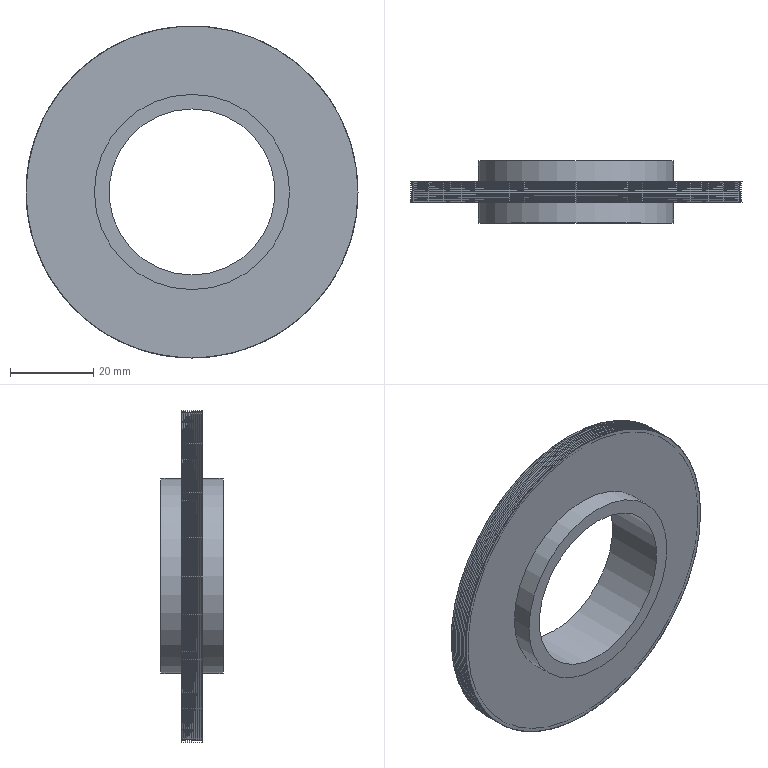Part | NX | features DATUM_CSYS 5, SKETCH 4, EXTRUDE 3, SWP104 1 | 1 solid | 41 faces | box 80 x 15 x 80 mm | volume 23126 mm3 | cone 22 | cylinder 15 | plane 4 | commonest cylinder face diameters 80 x12 47 x2 40 x1
STEP:
#1=CARTESIAN_POINT('',(40.,-10.,0.));
#2=VERTEX_POINT('',#1);
#3=CARTESIAN_POINT('',(0.,-10.,0.));
#4=DIRECTION('',(0.,1.,0.));
#5=DIRECTION('',(1.,0.,0.));
#6=AXIS2_PLACEMENT_3D('',#3,#4,#5);
#7=CIRCLE('',#6,40.);
#8=EDGE_CURVE('',#2,#2,#7,.T.);
#9=ORIENTED_EDGE('',*,*,#8,.T.);
#10=EDGE_LOOP('',(#9));
#11=FACE_BOUND('',#10,.T.);
#12=CARTESIAN_POINT('',(0.,-9.976,-40.));
#13=VERTEX_POINT('',#12);
#14=CARTESIAN_POINT('',(0.,-9.976,0.));
#15=DIRECTION('',(0.,-1.,0.));
#16=DIRECTION('',(0.,0.,-1.));
#17=AXIS2_PLACEMENT_3D('',#14,#15,#16);
#18=CIRCLE('',#17,40.);
#19=EDGE_CURVE('',#13,#13,#18,.T.);
#20=ORIENTED_EDGE('',*,*,#19,.T.);
#21=EDGE_LOOP('',(#20));
#22=FACE_BOUND('',#21,.T.);
#23=CARTESIAN_POINT('',(0.,-10.,0.));
#24=DIRECTION('',(0.,1.,0.));
#25=DIRECTION('',(0.,0.,1.));
#26=AXIS2_PLACEMENT_3D('',#23,#24,#25);
#27=CYLINDRICAL_SURFACE('',#26,40.);
#28=ADVANCED_FACE('',(#11,#22),#27,.T.);
#29=CARTESIAN_POINT('',(23.5,-15.,0.));
#30=VERTEX_POINT('',#29);
#31=CARTESIAN_POINT('',(0.,-15.,0.));
#32=DIRECTION('',(0.,-1.,0.));
#33=DIRECTION('',(1.,0.,0.));
#34=AXIS2_PLACEMENT_3D('',#31,#32,#33);
#35=CIRCLE('',#34,23.5);
#36=EDGE_CURVE('',#30,#30,#35,.T.);
#37=ORIENTED_EDGE('',*,*,#36,.F.);
#38=EDGE_LOOP('',(#37));
#39=FACE_BOUND('',#38,.T.);
#40=CARTESIAN_POINT('',(0.,-10.,23.5));
#41=VERTEX_POINT('',#40);
#42=CARTESIAN_POINT('',(0.,-10.,0.));
#43=DIRECTION('',(0.,1.,0.));
#44=DIRECTION('',(0.,0.,1.));
#45=AXIS2_PLACEMENT_3D('',#42,#43,#44);
#46=CIRCLE('',#45,23.5);
#47=EDGE_CURVE('',#41,#41,#46,.T.);
#48=ORIENTED_EDGE('',*,*,#47,.F.);
#49=EDGE_LOOP('',(#48));
#50=FACE_BOUND('',#49,.T.);
#51=CARTESIAN_POINT('',(0.,-15.,0.));
#52=DIRECTION('',(0.,1.,0.));
#53=DIRECTION('',(0.,0.,1.));
#54=AXIS2_PLACEMENT_3D('',#51,#52,#53);
#55=CYLINDRICAL_SURFACE('',#54,23.5);
#56=ADVANCED_FACE('',(#39,#50),#55,.T.);
#57=CARTESIAN_POINT('',(0.,-15.,-20.));
#58=VERTEX_POINT('',#57);
#59=CARTESIAN_POINT('',(0.,-15.,0.));
#60=DIRECTION('',(0.,-1.,0.));
#61=DIRECTION('',(0.,0.,-1.));
#62=AXIS2_PLACEMENT_3D('',#59,#60,#61);
#63=CIRCLE('',#62,20.);
#64=EDGE_CURVE('',#58,#58,#63,.F.);
#65=ORIENTED_EDGE('',*,*,#64,.T.);
#66=EDGE_LOOP('',(#65));
#67=FACE_BOUND('',#66,.T.);
#68=ORIENTED_EDGE('',*,*,#36,.T.);
#69=EDGE_LOOP('',(#68));
#70=FACE_BOUND('',#69,.T.);
#71=CARTESIAN_POINT('',(0.,-15.,0.));
#72=DIRECTION('',(0.,-1.,0.));
#73=DIRECTION('',(0.,0.,-1.));
#74=AXIS2_PLACEMENT_3D('',#71,#72,#73);
#75=PLANE('',#74);
#76=ADVANCED_FACE('',(#67,#70),#75,.T.);
#77=ORIENTED_EDGE('',*,*,#47,.T.);
#78=EDGE_LOOP('',(#77));
#79=FACE_BOUND('',#78,.T.);
#80=ORIENTED_EDGE('',*,*,#8,.F.);
#81=EDGE_LOOP('',(#80));
#82=FACE_BOUND('',#81,.T.);
#83=CARTESIAN_POINT('',(0.,-10.,0.));
#84=DIRECTION('',(0.,1.,0.));
#85=DIRECTION('',(0.,0.,1.));
#86=AXIS2_PLACEMENT_3D('',#83,#84,#85);
#87=PLANE('',#86);
#88=ADVANCED_FACE('',(#79,#82),#87,.F.);
#89=ORIENTED_EDGE('',*,*,#19,.F.);
#90=EDGE_LOOP('',(#89));
#91=FACE_BOUND('',#90,.T.);
#92=CARTESIAN_POINT('',(0.,-9.892,-39.157));
#93=VERTEX_POINT('',#92);
#94=CARTESIAN_POINT('',(0.,-9.892,0.));
#95=DIRECTION('',(0.,-1.,0.));
#96=DIRECTION('',(0.,0.,-1.));
#97=AXIS2_PLACEMENT_3D('',#94,#95,#96);
#98=CIRCLE('',#97,39.157);
#99=EDGE_CURVE('',#93,#93,#98,.F.);
#100=ORIENTED_EDGE('',*,*,#99,.F.);
#101=EDGE_LOOP('',(#100));
#102=FACE_BOUND('',#101,.T.);
#103=CARTESIAN_POINT('',(0.,-10.,0.));
#104=DIRECTION('',(0.,-1.,0.));
#105=DIRECTION('',(0.,0.,-1.));
#106=AXIS2_PLACEMENT_3D('',#103,#104,#105);
#107=CONICAL_SURFACE('',#106,40.237,1.471);
#108=ADVANCED_FACE('',(#91,#102),#107,.T.);
#109=CARTESIAN_POINT('',(0.,-9.682,40.));
#110=VERTEX_POINT('',#109);
#111=CARTESIAN_POINT('',(0.,-9.682,0.));
#112=DIRECTION('',(0.,1.,0.));
#113=DIRECTION('',(0.,0.,1.));
#114=AXIS2_PLACEMENT_3D('',#111,#112,#113);
#115=CIRCLE('',#114,40.);
#116=EDGE_CURVE('',#110,#110,#115,.T.);
#117=ORIENTED_EDGE('',*,*,#116,.F.);
#118=EDGE_LOOP('',(#117));
#119=FACE_BOUND('',#118,.T.);
#120=ORIENTED_EDGE('',*,*,#99,.T.);
#121=EDGE_LOOP('',(#120));
#122=FACE_BOUND('',#121,.T.);
#123=CARTESIAN_POINT('',(0.,-9.892,0.));
#124=DIRECTION('',(0.,1.,0.));
#125=DIRECTION('',(0.,0.,1.));
#126=AXIS2_PLACEMENT_3D('',#123,#124,#125);
#127=CONICAL_SURFACE('',#126,39.157,1.326);
#128=ADVANCED_FACE('',(#119,#122),#127,.T.);
#129=CARTESIAN_POINT('',(0.,-9.67,-40.));
#130=VERTEX_POINT('',#129);
#131=CARTESIAN_POINT('',(0.,-9.67,0.));
#132=DIRECTION('',(0.,-1.,0.));
#133=DIRECTION('',(0.,0.,-1.));
#134=AXIS2_PLACEMENT_3D('',#131,#132,#133);
#135=CIRCLE('',#134,40.);
#136=EDGE_CURVE('',#130,#130,#135,.T.);
#137=ORIENTED_EDGE('',*,*,#136,.T.);
#138=EDGE_LOOP('',(#137));
#139=FACE_BOUND('',#138,.T.);
#140=ORIENTED_EDGE('',*,*,#116,.T.);
#141=EDGE_LOOP('',(#140));
#142=FACE_BOUND('',#141,.T.);
#143=CARTESIAN_POINT('',(0.,-10.,0.));
#144=DIRECTION('',(0.,1.,0.));
#145=DIRECTION('',(0.,0.,1.));
#146=AXIS2_PLACEMENT_3D('',#143,#144,#145);
#147=CYLINDRICAL_SURFACE('',#146,40.);
#148=ADVANCED_FACE('',(#139,#142),#147,.T.);
#149=CARTESIAN_POINT('',(0.,-9.218,40.));
#150=VERTEX_POINT('',#149);
#151=CARTESIAN_POINT('',(0.,-9.218,0.));
#152=DIRECTION('',(0.,1.,0.));
#153=DIRECTION('',(0.,0.,1.));
#154=AXIS2_PLACEMENT_3D('',#151,#152,#153);
#155=CIRCLE('',#154,40.);
#156=EDGE_CURVE('',#150,#150,#155,.T.);
#157=ORIENTED_EDGE('',*,*,#156,.F.);
#158=EDGE_LOOP('',(#157));
#159=FACE_BOUND('',#158,.T.);
#160=CARTESIAN_POINT('',(0.,-9.428,-39.157));
#161=VERTEX_POINT('',#160);
#162=CARTESIAN_POINT('',(0.,-9.428,0.));
#163=DIRECTION('',(0.,-1.,0.));
#164=DIRECTION('',(0.,0.,-1.));
#165=AXIS2_PLACEMENT_3D('',#162,#163,#164);
#166=CIRCLE('',#165,39.157);
#167=EDGE_CURVE('',#161,#161,#166,.F.);
#168=ORIENTED_EDGE('',*,*,#167,.T.);
#169=EDGE_LOOP('',(#168));
#170=FACE_BOUND('',#169,.T.);
#171=CARTESIAN_POINT('',(0.,-9.428,0.));
#172=DIRECTION('',(0.,1.,0.));
#173=DIRECTION('',(0.,0.,1.));
#174=AXIS2_PLACEMENT_3D('',#171,#172,#173);
#175=CONICAL_SURFACE('',#174,39.157,1.326);
#176=ADVANCED_FACE('',(#159,#170),#175,.T.);
#177=ORIENTED_EDGE('',*,*,#136,.F.);
#178=EDGE_LOOP('',(#177));
#179=FACE_BOUND('',#178,.T.);
#180=ORIENTED_EDGE('',*,*,#167,.F.);
#181=EDGE_LOOP('',(#180));
#182=FACE_BOUND('',#181,.T.);
#183=CARTESIAN_POINT('',(0.,-9.676,0.));
#184=DIRECTION('',(0.,-1.,0.));
#185=DIRECTION('',(0.,0.,-1.));
#186=AXIS2_PLACEMENT_3D('',#183,#184,#185);
#187=CONICAL_SURFACE('',#186,40.022,1.292);
#188=ADVANCED_FACE('',(#179,#182),#187,.T.);
#189=CARTESIAN_POINT('',(0.,-9.206,-40.));
#190=VERTEX_POINT('',#189);
#191=CARTESIAN_POINT('',(0.,-9.206,0.));
#192=DIRECTION('',(0.,-1.,0.));
#193=DIRECTION('',(0.,0.,-1.));
#194=AXIS2_PLACEMENT_3D('',#191,#192,#193);
#195=CIRCLE('',#194,40.);
#196=EDGE_CURVE('',#190,#190,#195,.T.);
#197=ORIENTED_EDGE('',*,*,#196,.T.);
#198=EDGE_LOOP('',(#197));
#199=FACE_BOUND('',#198,.T.);
#200=ORIENTED_EDGE('',*,*,#156,.T.);
#201=EDGE_LOOP('',(#200));
#202=FACE_BOUND('',#201,.T.);
#203=CARTESIAN_POINT('',(0.,-10.,0.));
#204=DIRECTION('',(0.,1.,0.));
#205=DIRECTION('',(0.,0.,1.));
#206=AXIS2_PLACEMENT_3D('',#203,#204,#205);
#207=CYLINDRICAL_SURFACE('',#206,40.);
#208=ADVANCED_FACE('',(#199,#202),#207,.T.);
#209=CARTESIAN_POINT('',(0.,-8.754,40.));
#210=VERTEX_POINT('',#209);
#211=CARTESIAN_POINT('',(0.,-8.754,0.));
#212=DIRECTION('',(0.,1.,0.));
#213=DIRECTION('',(0.,0.,1.));
#214=AXIS2_PLACEMENT_3D('',#211,#212,#213);
#215=CIRCLE('',#214,40.);
#216=EDGE_CURVE('',#210,#210,#215,.T.);
#217=ORIENTED_EDGE('',*,*,#216,.F.);
#218=EDGE_LOOP('',(#217));
#219=FACE_BOUND('',#218,.T.);
#220=CARTESIAN_POINT('',(0.,-8.964,-39.157));
#221=VERTEX_POINT('',#220);
#222=CARTESIAN_POINT('',(0.,-8.964,0.));
#223=DIRECTION('',(0.,-1.,0.));
#224=DIRECTION('',(0.,0.,-1.));
#225=AXIS2_PLACEMENT_3D('',#222,#223,#224);
#226=CIRCLE('',#225,39.157);
#227=EDGE_CURVE('',#221,#221,#226,.F.);
#228=ORIENTED_EDGE('',*,*,#227,.T.);
#229=EDGE_LOOP('',(#228));
#230=FACE_BOUND('',#229,.T.);
#231=CARTESIAN_POINT('',(0.,-8.964,0.));
#232=DIRECTION('',(0.,1.,0.));
#233=DIRECTION('',(0.,0.,1.));
#234=AXIS2_PLACEMENT_3D('',#231,#232,#233);
#235=CONICAL_SURFACE('',#234,39.157,1.326);
#236=ADVANCED_FACE('',(#219,#230),#235,.T.);
#237=ORIENTED_EDGE('',*,*,#196,.F.);
#238=EDGE_LOOP('',(#237));
#239=FACE_BOUND('',#238,.T.);
#240=ORIENTED_EDGE('',*,*,#227,.F.);
#241=EDGE_LOOP('',(#240));
#242=FACE_BOUND('',#241,.T.);
#243=CARTESIAN_POINT('',(0.,-9.212,0.));
#244=DIRECTION('',(0.,-1.,0.));
#245=DIRECTION('',(0.,0.,-1.));
#246=AXIS2_PLACEMENT_3D('',#243,#244,#245);
#247=CONICAL_SURFACE('',#246,40.022,1.292);
#248=ADVANCED_FACE('',(#239,#242),#247,.T.);
#249=CARTESIAN_POINT('',(0.,-8.742,-40.));
#250=VERTEX_POINT('',#249);
#251=CARTESIAN_POINT('',(0.,-8.742,0.));
#252=DIRECTION('',(0.,-1.,0.));
#253=DIRECTION('',(0.,0.,-1.));
#254=AXIS2_PLACEMENT_3D('',#251,#252,#253);
#255=CIRCLE('',#254,40.);
#256=EDGE_CURVE('',#250,#250,#255,.T.);
#257=ORIENTED_EDGE('',*,*,#256,.T.);
#258=EDGE_LOOP('',(#257));
#259=FACE_BOUND('',#258,.T.);
#260=ORIENTED_EDGE('',*,*,#216,.T.);
#261=EDGE_LOOP('',(#260));
#262=FACE_BOUND('',#261,.T.);
#263=CARTESIAN_POINT('',(0.,-10.,0.));
#264=DIRECTION('',(0.,1.,0.));
#265=DIRECTION('',(0.,0.,1.));
#266=AXIS2_PLACEMENT_3D('',#263,#264,#265);
#267=CYLINDRICAL_SURFACE('',#266,40.);
#268=ADVANCED_FACE('',(#259,#262),#267,.T.);
#269=CARTESIAN_POINT('',(0.,-8.29,40.));
#270=VERTEX_POINT('',#269);
#271=CARTESIAN_POINT('',(0.,-8.29,0.));
#272=DIRECTION('',(0.,1.,0.));
#273=DIRECTION('',(0.,0.,1.));
#274=AXIS2_PLACEMENT_3D('',#271,#272,#273);
#275=CIRCLE('',#274,40.);
#276=EDGE_CURVE('',#270,#270,#275,.T.);
#277=ORIENTED_EDGE('',*,*,#276,.F.);
#278=EDGE_LOOP('',(#277));
#279=FACE_BOUND('',#278,.T.);
#280=CARTESIAN_POINT('',(0.,-8.5,-39.157));
#281=VERTEX_POINT('',#280);
#282=CARTESIAN_POINT('',(0.,-8.5,0.));
#283=DIRECTION('',(0.,-1.,0.));
#284=DIRECTION('',(0.,0.,-1.));
#285=AXIS2_PLACEMENT_3D('',#282,#283,#284);
#286=CIRCLE('',#285,39.157);
#287=EDGE_CURVE('',#281,#281,#286,.F.);
#288=ORIENTED_EDGE('',*,*,#287,.T.);
#289=EDGE_LOOP('',(#288));
#290=FACE_BOUND('',#289,.T.);
#291=CARTESIAN_POINT('',(0.,-8.5,0.));
#292=DIRECTION('',(0.,1.,0.));
#293=DIRECTION('',(0.,0.,1.));
#294=AXIS2_PLACEMENT_3D('',#291,#292,#293);
#295=CONICAL_SURFACE('',#294,39.157,1.326);
#296=ADVANCED_FACE('',(#279,#290),#295,.T.);
#297=ORIENTED_EDGE('',*,*,#256,.F.);
#298=EDGE_LOOP('',(#297));
#299=FACE_BOUND('',#298,.T.);
#300=ORIENTED_EDGE('',*,*,#287,.F.);
#301=EDGE_LOOP('',(#300));
#302=FACE_BOUND('',#301,.T.);
#303=CARTESIAN_POINT('',(0.,-8.749,0.));
#304=DIRECTION('',(0.,-1.,0.));
#305=DIRECTION('',(0.,0.,-1.));
#306=AXIS2_PLACEMENT_3D('',#303,#304,#305);
#307=CONICAL_SURFACE('',#306,40.022,1.292);
#308=ADVANCED_FACE('',(#299,#302),#307,.T.);
#309=CARTESIAN_POINT('',(0.,-8.278,-40.));
#310=VERTEX_POINT('',#309);
#311=CARTESIAN_POINT('',(0.,-8.278,0.));
#312=DIRECTION('',(0.,-1.,0.));
#313=DIRECTION('',(0.,0.,-1.));
#314=AXIS2_PLACEMENT_3D('',#311,#312,#313);
#315=CIRCLE('',#314,40.);
#316=EDGE_CURVE('',#310,#310,#315,.T.);
#317=ORIENTED_EDGE('',*,*,#316,.T.);
#318=EDGE_LOOP('',(#317));
#319=FACE_BOUND('',#318,.T.);
#320=ORIENTED_EDGE('',*,*,#276,.T.);
#321=EDGE_LOOP('',(#320));
#322=FACE_BOUND('',#321,.T.);
#323=CARTESIAN_POINT('',(0.,-10.,0.));
#324=DIRECTION('',(0.,1.,0.));
#325=DIRECTION('',(0.,0.,1.));
#326=AXIS2_PLACEMENT_3D('',#323,#324,#325);
#327=CYLINDRICAL_SURFACE('',#326,40.);
#328=ADVANCED_FACE('',(#319,#322),#327,.T.);
#329=CARTESIAN_POINT('',(0.,-7.826,40.));
#330=VERTEX_POINT('',#329);
#331=CARTESIAN_POINT('',(0.,-7.826,0.));
#332=DIRECTION('',(0.,1.,0.));
#333=DIRECTION('',(0.,0.,1.));
#334=AXIS2_PLACEMENT_3D('',#331,#332,#333);
#335=CIRCLE('',#334,40.);
#336=EDGE_CURVE('',#330,#330,#335,.T.);
#337=ORIENTED_EDGE('',*,*,#336,.F.);
#338=EDGE_LOOP('',(#337));
#339=FACE_BOUND('',#338,.T.);
#340=CARTESIAN_POINT('',(0.,-8.037,-39.157));
#341=VERTEX_POINT('',#340);
#342=CARTESIAN_POINT('',(0.,-8.037,0.));
#343=DIRECTION('',(0.,-1.,0.));
#344=DIRECTION('',(0.,0.,-1.));
#345=AXIS2_PLACEMENT_3D('',#342,#343,#344);
#346=CIRCLE('',#345,39.157);
#347=EDGE_CURVE('',#341,#341,#346,.F.);
#348=ORIENTED_EDGE('',*,*,#347,.T.);
#349=EDGE_LOOP('',(#348));
#350=FACE_BOUND('',#349,.T.);
#351=CARTESIAN_POINT('',(0.,-8.037,0.));
#352=DIRECTION('',(0.,1.,0.));
#353=DIRECTION('',(0.,0.,1.));
#354=AXIS2_PLACEMENT_3D('',#351,#352,#353);
#355=CONICAL_SURFACE('',#354,39.157,1.326);
#356=ADVANCED_FACE('',(#339,#350),#355,.T.);
#357=ORIENTED_EDGE('',*,*,#316,.F.);
#358=EDGE_LOOP('',(#357));
#359=FACE_BOUND('',#358,.T.);
#360=ORIENTED_EDGE('',*,*,#347,.F.);
#361=EDGE_LOOP('',(#360));
#362=FACE_BOUND('',#361,.T.);
#363=CARTESIAN_POINT('',(0.,-8.285,0.));
#364=DIRECTION('',(0.,-1.,0.));
#365=DIRECTION('',(0.,0.,-1.));
#366=AXIS2_PLACEMENT_3D('',#363,#364,#365);
#367=CONICAL_SURFACE('',#366,40.022,1.292);
#368=ADVANCED_FACE('',(#359,#362),#367,.T.);
#369=CARTESIAN_POINT('',(0.,-7.815,-40.));
#370=VERTEX_POINT('',#369);
#371=CARTESIAN_POINT('',(0.,-7.815,0.));
#372=DIRECTION('',(0.,-1.,0.));
#373=DIRECTION('',(0.,0.,-1.));
#374=AXIS2_PLACEMENT_3D('',#371,#372,#373);
#375=CIRCLE('',#374,40.);
#376=EDGE_CURVE('',#370,#370,#375,.T.);
#377=ORIENTED_EDGE('',*,*,#376,.T.);
#378=EDGE_LOOP('',(#377));
#379=FACE_BOUND('',#378,.T.);
#380=ORIENTED_EDGE('',*,*,#336,.T.);
#381=EDGE_LOOP('',(#380));
#382=FACE_BOUND('',#381,.T.);
#383=CARTESIAN_POINT('',(0.,-10.,0.));
#384=DIRECTION('',(0.,1.,0.));
#385=DIRECTION('',(0.,0.,1.));
#386=AXIS2_PLACEMENT_3D('',#383,#384,#385);
#387=CYLINDRICAL_SURFACE('',#386,40.);
#388=ADVANCED_FACE('',(#379,#382),#387,.T.);
#389=CARTESIAN_POINT('',(0.,-7.363,40.));
#390=VERTEX_POINT('',#389);
#391=CARTESIAN_POINT('',(0.,-7.363,0.));
#392=DIRECTION('',(0.,1.,0.));
#393=DIRECTION('',(0.,0.,1.));
#394=AXIS2_PLACEMENT_3D('',#391,#392,#393);
#395=CIRCLE('',#394,40.);
#396=EDGE_CURVE('',#390,#390,#395,.T.);
#397=ORIENTED_EDGE('',*,*,#396,.F.);
#398=EDGE_LOOP('',(#397));
#399=FACE_BOUND('',#398,.T.);
#400=CARTESIAN_POINT('',(0.,-7.573,-39.157));
#401=VERTEX_POINT('',#400);
#402=CARTESIAN_POINT('',(0.,-7.573,0.));
#403=DIRECTION('',(0.,-1.,0.));
#404=DIRECTION('',(0.,0.,-1.));
#405=AXIS2_PLACEMENT_3D('',#402,#403,#404);
#406=CIRCLE('',#405,39.157);
#407=EDGE_CURVE('',#401,#401,#406,.F.);
#408=ORIENTED_EDGE('',*,*,#407,.T.);
#409=EDGE_LOOP('',(#408));
#410=FACE_BOUND('',#409,.T.);
#411=CARTESIAN_POINT('',(0.,-7.573,0.));
#412=DIRECTION('',(0.,1.,0.));
#413=DIRECTION('',(0.,0.,1.));
#414=AXIS2_PLACEMENT_3D('',#411,#412,#413);
#415=CONICAL_SURFACE('',#414,39.157,1.326);
#416=ADVANCED_FACE('',(#399,#410),#415,.T.);
#417=ORIENTED_EDGE('',*,*,#376,.F.);
#418=EDGE_LOOP('',(#417));
#419=FACE_BOUND('',#418,.T.);
#420=ORIENTED_EDGE('',*,*,#407,.F.);
#421=EDGE_LOOP('',(#420));
#422=FACE_BOUND('',#421,.T.);
#423=CARTESIAN_POINT('',(0.,-7.821,0.));
#424=DIRECTION('',(0.,-1.,0.));
#425=DIRECTION('',(0.,0.,-1.));
#426=AXIS2_PLACEMENT_3D('',#423,#424,#425);
#427=CONICAL_SURFACE('',#426,40.022,1.292);
#428=ADVANCED_FACE('',(#419,#422),#427,.T.);
#429=CARTESIAN_POINT('',(0.,-7.351,-40.));
#430=VERTEX_POINT('',#429);
#431=CARTESIAN_POINT('',(0.,-7.351,0.));
#432=DIRECTION('',(0.,-1.,0.));
#433=DIRECTION('',(0.,0.,-1.));
#434=AXIS2_PLACEMENT_3D('',#431,#432,#433);
#435=CIRCLE('',#434,40.);
#436=EDGE_CURVE('',#430,#430,#435,.T.);
#437=ORIENTED_EDGE('',*,*,#436,.T.);
#438=EDGE_LOOP('',(#437));
#439=FACE_BOUND('',#438,.T.);
#440=ORIENTED_EDGE('',*,*,#396,.T.);
#441=EDGE_LOOP('',(#440));
#442=FACE_BOUND('',#441,.T.);
#443=CARTESIAN_POINT('',(0.,-10.,0.));
#444=DIRECTION('',(0.,1.,0.));
#445=DIRECTION('',(0.,0.,1.));
#446=AXIS2_PLACEMENT_3D('',#443,#444,#445);
#447=CYLINDRICAL_SURFACE('',#446,40.);
#448=ADVANCED_FACE('',(#439,#442),#447,.T.);
#449=CARTESIAN_POINT('',(0.,-6.899,40.));
#450=VERTEX_POINT('',#449);
#451=CARTESIAN_POINT('',(0.,-6.899,0.));
#452=DIRECTION('',(0.,1.,0.));
#453=DIRECTION('',(0.,0.,1.));
#454=AXIS2_PLACEMENT_3D('',#451,#452,#453);
#455=CIRCLE('',#454,40.);
#456=EDGE_CURVE('',#450,#450,#455,.T.);
#457=ORIENTED_EDGE('',*,*,#456,.F.);
#458=EDGE_LOOP('',(#457));
#459=FACE_BOUND('',#458,.T.);
#460=CARTESIAN_POINT('',(0.,-7.109,-39.157));
#461=VERTEX_POINT('',#460);
#462=CARTESIAN_POINT('',(0.,-7.109,0.));
#463=DIRECTION('',(0.,-1.,0.));
#464=DIRECTION('',(0.,0.,-1.));
#465=AXIS2_PLACEMENT_3D('',#462,#463,#464);
#466=CIRCLE('',#465,39.157);
#467=EDGE_CURVE('',#461,#461,#466,.F.);
#468=ORIENTED_EDGE('',*,*,#467,.T.);
#469=EDGE_LOOP('',(#468));
#470=FACE_BOUND('',#469,.T.);
#471=CARTESIAN_POINT('',(0.,-7.109,0.));
#472=DIRECTION('',(0.,1.,0.));
#473=DIRECTION('',(0.,0.,1.));
#474=AXIS2_PLACEMENT_3D('',#471,#472,#473);
#475=CONICAL_SURFACE('',#474,39.157,1.326);
#476=ADVANCED_FACE('',(#459,#470),#475,.T.);
#477=ORIENTED_EDGE('',*,*,#436,.F.);
#478=EDGE_LOOP('',(#477));
#479=FACE_BOUND('',#478,.T.);
#480=ORIENTED_EDGE('',*,*,#467,.F.);
#481=EDGE_LOOP('',(#480));
#482=FACE_BOUND('',#481,.T.);
#483=CARTESIAN_POINT('',(0.,-7.357,0.));
#484=DIRECTION('',(0.,-1.,0.));
#485=DIRECTION('',(0.,0.,-1.));
#486=AXIS2_PLACEMENT_3D('',#483,#484,#485);
#487=CONICAL_SURFACE('',#486,40.022,1.292);
#488=ADVANCED_FACE('',(#479,#482),#487,.T.);
#489=CARTESIAN_POINT('',(0.,-6.887,-40.));
#490=VERTEX_POINT('',#489);
#491=CARTESIAN_POINT('',(0.,-6.887,0.));
#492=DIRECTION('',(0.,-1.,0.));
#493=DIRECTION('',(0.,0.,-1.));
#494=AXIS2_PLACEMENT_3D('',#491,#492,#493);
#495=CIRCLE('',#494,40.);
#496=EDGE_CURVE('',#490,#490,#495,.T.);
#497=ORIENTED_EDGE('',*,*,#496,.T.);
#498=EDGE_LOOP('',(#497));
#499=FACE_BOUND('',#498,.T.);
#500=ORIENTED_EDGE('',*,*,#456,.T.);
#501=EDGE_LOOP('',(#500));
#502=FACE_BOUND('',#501,.T.);
#503=CARTESIAN_POINT('',(0.,-10.,0.));
#504=DIRECTION('',(0.,1.,0.));
#505=DIRECTION('',(0.,0.,1.));
#506=AXIS2_PLACEMENT_3D('',#503,#504,#505);
#507=CYLINDRICAL_SURFACE('',#506,40.);
#508=ADVANCED_FACE('',(#499,#502),#507,.T.);
#509=CARTESIAN_POINT('',(0.,-6.435,40.));
#510=VERTEX_POINT('',#509);
#511=CARTESIAN_POINT('',(0.,-6.435,0.));
#512=DIRECTION('',(0.,1.,0.));
#513=DIRECTION('',(0.,0.,1.));
#514=AXIS2_PLACEMENT_3D('',#511,#512,#513);
#515=CIRCLE('',#514,40.);
#516=EDGE_CURVE('',#510,#510,#515,.T.);
#517=ORIENTED_EDGE('',*,*,#516,.F.);
#518=EDGE_LOOP('',(#517));
#519=FACE_BOUND('',#518,.T.);
#520=CARTESIAN_POINT('',(0.,-6.645,-39.157));
#521=VERTEX_POINT('',#520);
#522=CARTESIAN_POINT('',(0.,-6.645,0.));
#523=DIRECTION('',(0.,-1.,0.));
#524=DIRECTION('',(0.,0.,-1.));
#525=AXIS2_PLACEMENT_3D('',#522,#523,#524);
#526=CIRCLE('',#525,39.157);
#527=EDGE_CURVE('',#521,#521,#526,.F.);
#528=ORIENTED_EDGE('',*,*,#527,.T.);
#529=EDGE_LOOP('',(#528));
#530=FACE_BOUND('',#529,.T.);
#531=CARTESIAN_POINT('',(0.,-6.645,0.));
#532=DIRECTION('',(0.,1.,0.));
#533=DIRECTION('',(0.,0.,1.));
#534=AXIS2_PLACEMENT_3D('',#531,#532,#533);
#535=CONICAL_SURFACE('',#534,39.157,1.326);
#536=ADVANCED_FACE('',(#519,#530),#535,.T.);
#537=ORIENTED_EDGE('',*,*,#496,.F.);
#538=EDGE_LOOP('',(#537));
#539=FACE_BOUND('',#538,.T.);
#540=ORIENTED_EDGE('',*,*,#527,.F.);
#541=EDGE_LOOP('',(#540));
#542=FACE_BOUND('',#541,.T.);
#543=CARTESIAN_POINT('',(0.,-6.893,0.));
#544=DIRECTION('',(0.,-1.,0.));
#545=DIRECTION('',(0.,0.,-1.));
#546=AXIS2_PLACEMENT_3D('',#543,#544,#545);
#547=CONICAL_SURFACE('',#546,40.022,1.292);
#548=ADVANCED_FACE('',(#539,#542),#547,.T.);
#549=CARTESIAN_POINT('',(0.,-6.423,-40.));
#550=VERTEX_POINT('',#549);
#551=CARTESIAN_POINT('',(0.,-6.423,0.));
#552=DIRECTION('',(0.,-1.,0.));
#553=DIRECTION('',(0.,0.,-1.));
#554=AXIS2_PLACEMENT_3D('',#551,#552,#553);
#555=CIRCLE('',#554,40.);
#556=EDGE_CURVE('',#550,#550,#555,.T.);
#557=ORIENTED_EDGE('',*,*,#556,.T.);
#558=EDGE_LOOP('',(#557));
#559=FACE_BOUND('',#558,.T.);
#560=ORIENTED_EDGE('',*,*,#516,.T.);
#561=EDGE_LOOP('',(#560));
#562=FACE_BOUND('',#561,.T.);
#563=CARTESIAN_POINT('',(0.,-10.,0.));
#564=DIRECTION('',(0.,1.,0.));
#565=DIRECTION('',(0.,0.,1.));
#566=AXIS2_PLACEMENT_3D('',#563,#564,#565);
#567=CYLINDRICAL_SURFACE('',#566,40.);
#568=ADVANCED_FACE('',(#559,#562),#567,.T.);
#569=CARTESIAN_POINT('',(0.,-5.971,40.));
#570=VERTEX_POINT('',#569);
#571=CARTESIAN_POINT('',(0.,-5.971,0.));
#572=DIRECTION('',(0.,1.,0.));
#573=DIRECTION('',(0.,0.,1.));
#574=AXIS2_PLACEMENT_3D('',#571,#572,#573);
#575=CIRCLE('',#574,40.);
#576=EDGE_CURVE('',#570,#570,#575,.T.);
#577=ORIENTED_EDGE('',*,*,#576,.F.);
#578=EDGE_LOOP('',(#577));
#579=FACE_BOUND('',#578,.T.);
#580=CARTESIAN_POINT('',(0.,-6.182,-39.157));
#581=VERTEX_POINT('',#580);
#582=CARTESIAN_POINT('',(0.,-6.182,0.));
#583=DIRECTION('',(0.,-1.,0.));
#584=DIRECTION('',(0.,0.,-1.));
#585=AXIS2_PLACEMENT_3D('',#582,#583,#584);
#586=CIRCLE('',#585,39.157);
#587=EDGE_CURVE('',#581,#581,#586,.F.);
#588=ORIENTED_EDGE('',*,*,#587,.T.);
#589=EDGE_LOOP('',(#588));
#590=FACE_BOUND('',#589,.T.);
#591=CARTESIAN_POINT('',(0.,-6.182,0.));
#592=DIRECTION('',(0.,1.,0.));
#593=DIRECTION('',(0.,0.,1.));
#594=AXIS2_PLACEMENT_3D('',#591,#592,#593);
#595=CONICAL_SURFACE('',#594,39.157,1.326);
#596=ADVANCED_FACE('',(#579,#590),#595,.T.);
#597=ORIENTED_EDGE('',*,*,#556,.F.);
#598=EDGE_LOOP('',(#597));
#599=FACE_BOUND('',#598,.T.);
#600=ORIENTED_EDGE('',*,*,#587,.F.);
#601=EDGE_LOOP('',(#600));
#602=FACE_BOUND('',#601,.T.);
#603=CARTESIAN_POINT('',(0.,-6.43,0.));
#604=DIRECTION('',(0.,-1.,0.));
#605=DIRECTION('',(0.,0.,-1.));
#606=AXIS2_PLACEMENT_3D('',#603,#604,#605);
#607=CONICAL_SURFACE('',#606,40.022,1.292);
#608=ADVANCED_FACE('',(#599,#602),#607,.T.);
#609=CARTESIAN_POINT('',(0.,-5.96,-40.));
#610=VERTEX_POINT('',#609);
#611=CARTESIAN_POINT('',(0.,-5.96,0.));
#612=DIRECTION('',(0.,-1.,0.));
#613=DIRECTION('',(0.,0.,-1.));
#614=AXIS2_PLACEMENT_3D('',#611,#612,#613);
#615=CIRCLE('',#614,40.);
#616=EDGE_CURVE('',#610,#610,#615,.T.);
#617=ORIENTED_EDGE('',*,*,#616,.T.);
#618=EDGE_LOOP('',(#617));
#619=FACE_BOUND('',#618,.T.);
#620=ORIENTED_EDGE('',*,*,#576,.T.);
#621=EDGE_LOOP('',(#620));
#622=FACE_BOUND('',#621,.T.);
#623=CARTESIAN_POINT('',(0.,-10.,0.));
#624=DIRECTION('',(0.,1.,0.));
#625=DIRECTION('',(0.,0.,1.));
#626=AXIS2_PLACEMENT_3D('',#623,#624,#625);
#627=CYLINDRICAL_SURFACE('',#626,40.);
#628=ADVANCED_FACE('',(#619,#622),#627,.T.);
#629=CARTESIAN_POINT('',(0.,-5.508,40.));
#630=VERTEX_POINT('',#629);
#631=CARTESIAN_POINT('',(0.,-5.508,0.));
#632=DIRECTION('',(0.,1.,0.));
#633=DIRECTION('',(0.,0.,1.));
#634=AXIS2_PLACEMENT_3D('',#631,#632,#633);
#635=CIRCLE('',#634,40.);
#636=EDGE_CURVE('',#630,#630,#635,.T.);
#637=ORIENTED_EDGE('',*,*,#636,.F.);
#638=EDGE_LOOP('',(#637));
#639=FACE_BOUND('',#638,.T.);
#640=CARTESIAN_POINT('',(0.,-5.718,-39.157));
#641=VERTEX_POINT('',#640);
#642=CARTESIAN_POINT('',(0.,-5.718,0.));
#643=DIRECTION('',(0.,-1.,0.));
#644=DIRECTION('',(0.,0.,-1.));
#645=AXIS2_PLACEMENT_3D('',#642,#643,#644);
#646=CIRCLE('',#645,39.157);
#647=EDGE_CURVE('',#641,#641,#646,.F.);
#648=ORIENTED_EDGE('',*,*,#647,.T.);
#649=EDGE_LOOP('',(#648));
#650=FACE_BOUND('',#649,.T.);
#651=CARTESIAN_POINT('',(0.,-5.718,0.));
#652=DIRECTION('',(0.,1.,0.));
#653=DIRECTION('',(0.,0.,1.));
#654=AXIS2_PLACEMENT_3D('',#651,#652,#653);
#655=CONICAL_SURFACE('',#654,39.157,1.326);
#656=ADVANCED_FACE('',(#639,#650),#655,.T.);
#657=ORIENTED_EDGE('',*,*,#616,.F.);
#658=EDGE_LOOP('',(#657));
#659=FACE_BOUND('',#658,.T.);
#660=ORIENTED_EDGE('',*,*,#647,.F.);
#661=EDGE_LOOP('',(#660));
#662=FACE_BOUND('',#661,.T.);
#663=CARTESIAN_POINT('',(0.,-5.966,0.));
#664=DIRECTION('',(0.,-1.,0.));
#665=DIRECTION('',(0.,0.,-1.));
#666=AXIS2_PLACEMENT_3D('',#663,#664,#665);
#667=CONICAL_SURFACE('',#666,40.022,1.292);
#668=ADVANCED_FACE('',(#659,#662),#667,.T.);
#669=CARTESIAN_POINT('',(0.,-5.496,-40.));
#670=VERTEX_POINT('',#669);
#671=CARTESIAN_POINT('',(0.,-5.496,0.));
#672=DIRECTION('',(0.,-1.,0.));
#673=DIRECTION('',(0.,0.,-1.));
#674=AXIS2_PLACEMENT_3D('',#671,#672,#673);
#675=CIRCLE('',#674,40.);
#676=EDGE_CURVE('',#670,#670,#675,.T.);
#677=ORIENTED_EDGE('',*,*,#676,.T.);
#678=EDGE_LOOP('',(#677));
#679=FACE_BOUND('',#678,.T.);
#680=ORIENTED_EDGE('',*,*,#636,.T.);
#681=EDGE_LOOP('',(#680));
#682=FACE_BOUND('',#681,.T.);
#683=CARTESIAN_POINT('',(0.,-10.,0.));
#684=DIRECTION('',(0.,1.,0.));
#685=DIRECTION('',(0.,0.,1.));
#686=AXIS2_PLACEMENT_3D('',#683,#684,#685);
#687=CYLINDRICAL_SURFACE('',#686,40.);
#688=ADVANCED_FACE('',(#679,#682),#687,.T.);
#689=CARTESIAN_POINT('',(0.,-5.044,40.));
#690=VERTEX_POINT('',#689);
#691=CARTESIAN_POINT('',(0.,-5.044,0.));
#692=DIRECTION('',(0.,1.,0.));
#693=DIRECTION('',(0.,0.,1.));
#694=AXIS2_PLACEMENT_3D('',#691,#692,#693);
#695=CIRCLE('',#694,40.);
#696=EDGE_CURVE('',#690,#690,#695,.T.);
#697=ORIENTED_EDGE('',*,*,#696,.F.);
#698=EDGE_LOOP('',(#697));
#699=FACE_BOUND('',#698,.T.);
#700=CARTESIAN_POINT('',(0.,-5.254,-39.157));
#701=VERTEX_POINT('',#700);
#702=CARTESIAN_POINT('',(0.,-5.254,0.));
#703=DIRECTION('',(0.,-1.,0.));
#704=DIRECTION('',(0.,0.,-1.));
#705=AXIS2_PLACEMENT_3D('',#702,#703,#704);
#706=CIRCLE('',#705,39.157);
#707=EDGE_CURVE('',#701,#701,#706,.F.);
#708=ORIENTED_EDGE('',*,*,#707,.T.);
#709=EDGE_LOOP('',(#708));
#710=FACE_BOUND('',#709,.T.);
#711=CARTESIAN_POINT('',(0.,-5.254,0.));
#712=DIRECTION('',(0.,1.,0.));
#713=DIRECTION('',(0.,0.,1.));
#714=AXIS2_PLACEMENT_3D('',#711,#712,#713);
#715=CONICAL_SURFACE('',#714,39.157,1.326);
#716=ADVANCED_FACE('',(#699,#710),#715,.T.);
#717=ORIENTED_EDGE('',*,*,#676,.F.);
#718=EDGE_LOOP('',(#717));
#719=FACE_BOUND('',#718,.T.);
#720=ORIENTED_EDGE('',*,*,#707,.F.);
#721=EDGE_LOOP('',(#720));
#722=FACE_BOUND('',#721,.T.);
#723=CARTESIAN_POINT('',(0.,-5.502,0.));
#724=DIRECTION('',(0.,-1.,0.));
#725=DIRECTION('',(0.,0.,-1.));
#726=AXIS2_PLACEMENT_3D('',#723,#724,#725);
#727=CONICAL_SURFACE('',#726,40.022,1.292);
#728=ADVANCED_FACE('',(#719,#722),#727,.T.);
#729=CARTESIAN_POINT('',(0.,0.,-20.));
#730=VERTEX_POINT('',#729);
#731=CARTESIAN_POINT('',(0.,0.,0.));
#732=DIRECTION('',(0.,-1.,0.));
#733=DIRECTION('',(0.,0.,-1.));
#734=AXIS2_PLACEMENT_3D('',#731,#732,#733);
#735=CIRCLE('',#734,20.);
#736=EDGE_CURVE('',#730,#730,#735,.F.);
#737=ORIENTED_EDGE('',*,*,#736,.F.);
#738=EDGE_LOOP('',(#737));
#739=FACE_BOUND('',#738,.T.);
#740=CARTESIAN_POINT('',(23.5,0.,0.));
#741=VERTEX_POINT('',#740);
#742=CARTESIAN_POINT('',(0.,0.,0.));
#743=DIRECTION('',(0.,-1.,0.));
#744=DIRECTION('',(1.,0.,0.));
#745=AXIS2_PLACEMENT_3D('',#742,#743,#744);
#746=CIRCLE('',#745,23.5);
#747=EDGE_CURVE('',#741,#741,#746,.T.);
#748=ORIENTED_EDGE('',*,*,#747,.F.);
#749=EDGE_LOOP('',(#748));
#750=FACE_BOUND('',#749,.T.);
#751=CARTESIAN_POINT('',(0.,0.,0.));
#752=DIRECTION('',(0.,-1.,0.));
#753=DIRECTION('',(0.,0.,-1.));
#754=AXIS2_PLACEMENT_3D('',#751,#752,#753);
#755=PLANE('',#754);
#756=ADVANCED_FACE('',(#739,#750),#755,.F.);
#757=CARTESIAN_POINT('',(0.,-5.,23.5));
#758=VERTEX_POINT('',#757);
#759=CARTESIAN_POINT('',(0.,-5.,0.));
#760=DIRECTION('',(0.,1.,0.));
#761=DIRECTION('',(0.,0.,1.));
#762=AXIS2_PLACEMENT_3D('',#759,#760,#761);
#763=CIRCLE('',#762,23.5);
#764=EDGE_CURVE('',#758,#758,#763,.T.);
#765=ORIENTED_EDGE('',*,*,#764,.T.);
#766=EDGE_LOOP('',(#765));
#767=FACE_BOUND('',#766,.T.);
#768=ORIENTED_EDGE('',*,*,#747,.T.);
#769=EDGE_LOOP('',(#768));
#770=FACE_BOUND('',#769,.T.);
#771=CARTESIAN_POINT('',(0.,-15.,0.));
#772=DIRECTION('',(0.,1.,0.));
#773=DIRECTION('',(0.,0.,1.));
#774=AXIS2_PLACEMENT_3D('',#771,#772,#773);
#775=CYLINDRICAL_SURFACE('',#774,23.5);
#776=ADVANCED_FACE('',(#767,#770),#775,.T.);
#777=ORIENTED_EDGE('',*,*,#764,.F.);
#778=EDGE_LOOP('',(#777));
#779=FACE_BOUND('',#778,.T.);
#780=CARTESIAN_POINT('',(40.,-5.,0.));
#781=VERTEX_POINT('',#780);
#782=CARTESIAN_POINT('',(0.,-5.,0.));
#783=DIRECTION('',(0.,1.,0.));
#784=DIRECTION('',(1.,0.,0.));
#785=AXIS2_PLACEMENT_3D('',#782,#783,#784);
#786=CIRCLE('',#785,40.);
#787=EDGE_CURVE('',#781,#781,#786,.T.);
#788=ORIENTED_EDGE('',*,*,#787,.T.);
#789=EDGE_LOOP('',(#788));
#790=FACE_BOUND('',#789,.T.);
#791=CARTESIAN_POINT('',(0.,-5.,0.));
#792=DIRECTION('',(0.,1.,0.));
#793=DIRECTION('',(0.,0.,1.));
#794=AXIS2_PLACEMENT_3D('',#791,#792,#793);
#795=PLANE('',#794);
#796=ADVANCED_FACE('',(#779,#790),#795,.T.);
#797=ORIENTED_EDGE('',*,*,#787,.F.);
#798=EDGE_LOOP('',(#797));
#799=FACE_BOUND('',#798,.T.);
#800=ORIENTED_EDGE('',*,*,#696,.T.);
#801=EDGE_LOOP('',(#800));
#802=FACE_BOUND('',#801,.T.);
#803=CARTESIAN_POINT('',(0.,-10.,0.));
#804=DIRECTION('',(0.,1.,0.));
#805=DIRECTION('',(0.,0.,1.));
#806=AXIS2_PLACEMENT_3D('',#803,#804,#805);
#807=CYLINDRICAL_SURFACE('',#806,40.);
#808=ADVANCED_FACE('',(#799,#802),#807,.T.);
#809=ORIENTED_EDGE('',*,*,#64,.F.);
#810=EDGE_LOOP('',(#809));
#811=FACE_BOUND('',#810,.T.);
#812=ORIENTED_EDGE('',*,*,#736,.T.);
#813=EDGE_LOOP('',(#812));
#814=FACE_BOUND('',#813,.T.);
#815=CARTESIAN_POINT('',(0.,10.,0.));
#816=DIRECTION('',(0.,-1.,0.));
#817=DIRECTION('',(0.,0.,-1.));
#818=AXIS2_PLACEMENT_3D('',#815,#816,#817);
#819=CYLINDRICAL_SURFACE('',#818,20.);
#820=ADVANCED_FACE('',(#811,#814),#819,.F.);
#821=CLOSED_SHELL('',(#28,#56,#76,#88,#108,#128,#148,#176,#188,#208,#236,#248,#268,#296,#308,#328,#356,#368,#388,#416,#428,#448,#476,#488,#508,#536,#548,#568,#596,#608,#628,#656,#668,#688,#716,#728,#756,#776,#796,#808,#820));
#822=MANIFOLD_SOLID_BREP('',#821);
#823=(LENGTH_UNIT()NAMED_UNIT(*)SI_UNIT(.MILLI.,.METRE.));
#824=UNCERTAINTY_MEASURE_WITH_UNIT(LENGTH_MEASURE(0.00001),#823,'','');
#825=(NAMED_UNIT(*)PLANE_ANGLE_UNIT()SI_UNIT($,.RADIAN.));
#826=(NAMED_UNIT(*)SI_UNIT($,.STERADIAN.)SOLID_ANGLE_UNIT());
#827=(GEOMETRIC_REPRESENTATION_CONTEXT(3)GLOBAL_UNCERTAINTY_ASSIGNED_CONTEXT((#824))GLOBAL_UNIT_ASSIGNED_CONTEXT((#823,#825,#826))REPRESENTATION_CONTEXT('',''));
#828=ADVANCED_BREP_SHAPE_REPRESENTATION('',(#822),#827);